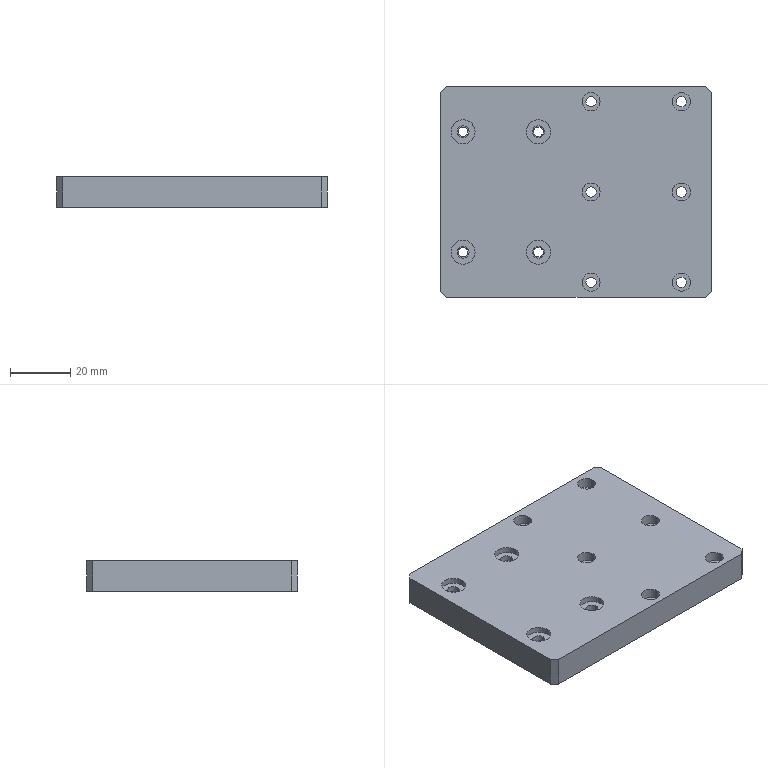Part | SolidWorks | features HoleWzd 2, ICE 2, Chamfer 1, Extrusion 1 | 1 solid | 84 faces | box 90 x 70 x 10 mm | volume 61013 mm3 | cylinder 56 | plane 28 | commonest cylinder face diameters 6 x20 3.4 x12 3.2 x8 4 x8 8 x8